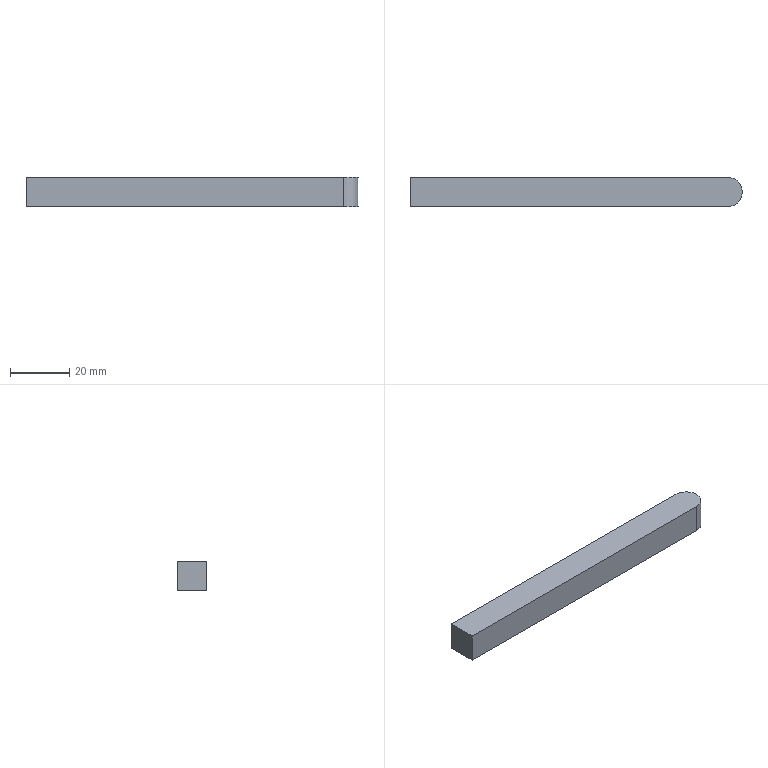Part | NX | features solid 2 | 1 solid | 6 faces | box 112.5 x 10 x 10 mm | volume 11143 mm3 | plane 5 | cylinder 1 | commonest cylinder face diameters 10 x1
STEP:
#1=CARTESIAN_POINT('',(15.,722.5,-125.));
#2=VERTEX_POINT('',#1);
#3=CARTESIAN_POINT('',(15.,722.5,-115.));
#4=VERTEX_POINT('',#3);
#5=CARTESIAN_POINT('',(15.,722.5,-115.));
#6=DIRECTION('',(0.,0.,1.));
#7=VECTOR('',#6,1000.);
#8=LINE('',#5,#7);
#9=EDGE_CURVE('',#2,#4,#8,.T.);
#10=ORIENTED_EDGE('',*,*,#9,.T.);
#11=CARTESIAN_POINT('',(122.5,722.5,-115.));
#12=VERTEX_POINT('',#11);
#13=CARTESIAN_POINT('',(-10.,722.5,-115.));
#14=DIRECTION('',(-1.,0.,0.));
#15=VECTOR('',#14,1000.);
#16=LINE('',#13,#15);
#17=EDGE_CURVE('',#12,#4,#16,.T.);
#18=ORIENTED_EDGE('',*,*,#17,.F.);
#19=CARTESIAN_POINT('',(122.5,722.5,-125.));
#20=VERTEX_POINT('',#19);
#21=CARTESIAN_POINT('',(122.5,722.5,-115.));
#22=DIRECTION('',(0.,0.,-1.));
#23=VECTOR('',#22,1000.);
#24=LINE('',#21,#23);
#25=EDGE_CURVE('',#12,#20,#24,.T.);
#26=ORIENTED_EDGE('',*,*,#25,.T.);
#27=CARTESIAN_POINT('',(-10.,722.5,-125.));
#28=DIRECTION('',(-1.,0.,0.));
#29=VECTOR('',#28,1000.);
#30=LINE('',#27,#29);
#31=EDGE_CURVE('',#20,#2,#30,.T.);
#32=ORIENTED_EDGE('',*,*,#31,.T.);
#33=EDGE_LOOP('',(#10,#18,#26,#32));
#34=FACE_BOUND('',#33,.T.);
#35=CARTESIAN_POINT('',(130.,722.5,-115.));
#36=DIRECTION('',(0.,1.,0.));
#37=DIRECTION('',(0.,0.,1.));
#38=AXIS2_PLACEMENT_3D('',#35,#36,#37);
#39=PLANE('',#38);
#40=ADVANCED_FACE('',(#34),#39,.T.);
#41=CARTESIAN_POINT('',(122.5,712.5,-125.));
#42=VERTEX_POINT('',#41);
#43=CARTESIAN_POINT('',(122.5,717.5,-125.));
#44=DIRECTION('',(0.,0.,1.));
#45=DIRECTION('',(1.,0.,0.));
#46=AXIS2_PLACEMENT_3D('',#43,#44,#45);
#47=CIRCLE('',#46,5.);
#48=EDGE_CURVE('',#42,#20,#47,.T.);
#49=ORIENTED_EDGE('',*,*,#48,.T.);
#50=ORIENTED_EDGE('',*,*,#25,.F.);
#51=CARTESIAN_POINT('',(122.5,712.5,-115.));
#52=VERTEX_POINT('',#51);
#53=CARTESIAN_POINT('',(122.5,717.5,-115.));
#54=DIRECTION('',(0.,0.,1.));
#55=DIRECTION('',(1.,0.,0.));
#56=AXIS2_PLACEMENT_3D('',#53,#54,#55);
#57=CIRCLE('',#56,5.);
#58=EDGE_CURVE('',#52,#12,#57,.T.);
#59=ORIENTED_EDGE('',*,*,#58,.F.);
#60=CARTESIAN_POINT('',(122.5,712.5,-115.));
#61=DIRECTION('',(0.,0.,-1.));
#62=VECTOR('',#61,1000.);
#63=LINE('',#60,#62);
#64=EDGE_CURVE('',#52,#42,#63,.T.);
#65=ORIENTED_EDGE('',*,*,#64,.T.);
#66=EDGE_LOOP('',(#49,#50,#59,#65));
#67=FACE_BOUND('',#66,.T.);
#68=CARTESIAN_POINT('',(122.5,717.5,-115.));
#69=DIRECTION('',(0.,0.,-1.));
#70=DIRECTION('',(1.,0.,0.));
#71=AXIS2_PLACEMENT_3D('',#68,#69,#70);
#72=CYLINDRICAL_SURFACE('',#71,5.);
#73=ADVANCED_FACE('',(#67),#72,.T.);
#74=CARTESIAN_POINT('',(15.,712.5,-115.));
#75=VERTEX_POINT('',#74);
#76=CARTESIAN_POINT('',(15.,712.5,-125.));
#77=VERTEX_POINT('',#76);
#78=CARTESIAN_POINT('',(15.,712.5,-115.));
#79=DIRECTION('',(0.,0.,-1.));
#80=VECTOR('',#79,1000.);
#81=LINE('',#78,#80);
#82=EDGE_CURVE('',#75,#77,#81,.T.);
#83=ORIENTED_EDGE('',*,*,#82,.T.);
#84=CARTESIAN_POINT('',(-10.,712.5,-125.));
#85=DIRECTION('',(1.,0.,0.));
#86=VECTOR('',#85,1000.);
#87=LINE('',#84,#86);
#88=EDGE_CURVE('',#77,#42,#87,.T.);
#89=ORIENTED_EDGE('',*,*,#88,.T.);
#90=ORIENTED_EDGE('',*,*,#64,.F.);
#91=CARTESIAN_POINT('',(-10.,712.5,-115.));
#92=DIRECTION('',(1.,0.,0.));
#93=VECTOR('',#92,1000.);
#94=LINE('',#91,#93);
#95=EDGE_CURVE('',#75,#52,#94,.T.);
#96=ORIENTED_EDGE('',*,*,#95,.F.);
#97=EDGE_LOOP('',(#83,#89,#90,#96));
#98=FACE_BOUND('',#97,.T.);
#99=CARTESIAN_POINT('',(-10.,712.5,-115.));
#100=DIRECTION('',(0.,-1.,0.));
#101=DIRECTION('',(0.,0.,-1.));
#102=AXIS2_PLACEMENT_3D('',#99,#100,#101);
#103=PLANE('',#102);
#104=ADVANCED_FACE('',(#98),#103,.T.);
#105=ORIENTED_EDGE('',*,*,#95,.T.);
#106=ORIENTED_EDGE('',*,*,#58,.T.);
#107=ORIENTED_EDGE('',*,*,#17,.T.);
#108=CARTESIAN_POINT('',(15.,725.,-115.));
#109=DIRECTION('',(0.,1.,0.));
#110=VECTOR('',#109,1000.);
#111=LINE('',#108,#110);
#112=EDGE_CURVE('',#75,#4,#111,.T.);
#113=ORIENTED_EDGE('',*,*,#112,.F.);
#114=EDGE_LOOP('',(#105,#106,#107,#113));
#115=FACE_BOUND('',#114,.T.);
#116=CARTESIAN_POINT('',(-10.,725.,-115.));
#117=DIRECTION('',(0.,0.,-1.));
#118=DIRECTION('',(1.,0.,0.));
#119=AXIS2_PLACEMENT_3D('',#116,#117,#118);
#120=PLANE('',#119);
#121=ADVANCED_FACE('',(#115),#120,.F.);
#122=CARTESIAN_POINT('',(15.,725.,-125.));
#123=DIRECTION('',(0.,1.,0.));
#124=VECTOR('',#123,1000.);
#125=LINE('',#122,#124);
#126=EDGE_CURVE('',#77,#2,#125,.T.);
#127=ORIENTED_EDGE('',*,*,#126,.T.);
#128=ORIENTED_EDGE('',*,*,#31,.F.);
#129=ORIENTED_EDGE('',*,*,#48,.F.);
#130=ORIENTED_EDGE('',*,*,#88,.F.);
#131=EDGE_LOOP('',(#127,#128,#129,#130));
#132=FACE_BOUND('',#131,.T.);
#133=CARTESIAN_POINT('',(-10.,725.,-125.));
#134=DIRECTION('',(0.,0.,-1.));
#135=DIRECTION('',(1.,0.,0.));
#136=AXIS2_PLACEMENT_3D('',#133,#134,#135);
#137=PLANE('',#136);
#138=ADVANCED_FACE('',(#132),#137,.T.);
#139=ORIENTED_EDGE('',*,*,#112,.T.);
#140=ORIENTED_EDGE('',*,*,#9,.F.);
#141=ORIENTED_EDGE('',*,*,#126,.F.);
#142=ORIENTED_EDGE('',*,*,#82,.F.);
#143=EDGE_LOOP('',(#139,#140,#141,#142));
#144=FACE_BOUND('',#143,.T.);
#145=CARTESIAN_POINT('',(15.,722.5,-115.));
#146=DIRECTION('',(1.,0.,0.));
#147=DIRECTION('',(0.,0.,1.));
#148=AXIS2_PLACEMENT_3D('',#145,#146,#147);
#149=PLANE('',#148);
#150=ADVANCED_FACE('',(#144),#149,.F.);
#151=CLOSED_SHELL('',(#40,#73,#104,#121,#138,#150));
#152=MANIFOLD_SOLID_BREP('',#151);
#153=(LENGTH_UNIT()NAMED_UNIT(*)SI_UNIT(.MILLI.,.METRE.));
#154=UNCERTAINTY_MEASURE_WITH_UNIT(LENGTH_MEASURE(0.00001),#153,'','');
#155=(NAMED_UNIT(*)PLANE_ANGLE_UNIT()SI_UNIT($,.RADIAN.));
#156=(NAMED_UNIT(*)SI_UNIT($,.STERADIAN.)SOLID_ANGLE_UNIT());
#157=(GEOMETRIC_REPRESENTATION_CONTEXT(3)GLOBAL_UNCERTAINTY_ASSIGNED_CONTEXT((#154))GLOBAL_UNIT_ASSIGNED_CONTEXT((#153,#155,#156))REPRESENTATION_CONTEXT('',''));
#158=ADVANCED_BREP_SHAPE_REPRESENTATION('',(#152),#157);